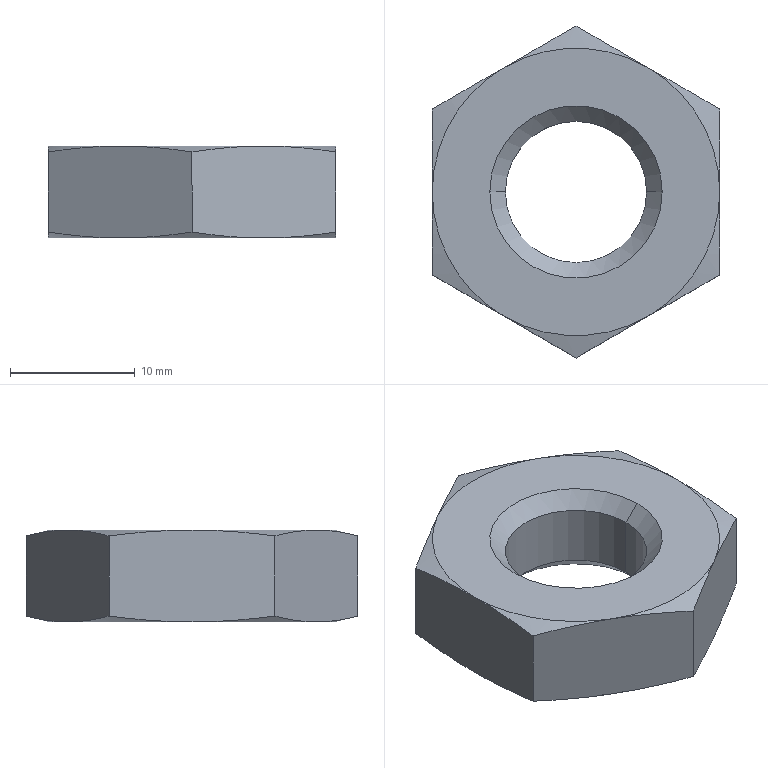Part | SolidWorks | features BaseBody 1 | 1 solid | 26 faces | box 23.077 x 26.647 x 7.385 mm | volume 2587 mm3 | cone 16 | plane 8 | cylinder 2 | commonest cylinder face diameters 11.347 x2
STEP:
#1=CARTESIAN_POINT('',(-12.08,360.269,293.557));
#2=VERTEX_POINT('',#1);
#3=CARTESIAN_POINT('',(-23.427,360.269,293.557));
#4=VERTEX_POINT('',#3);
#5=CARTESIAN_POINT('',(-17.753,360.269,293.557));
#6=DIRECTION('',(0.,0.,-1.));
#7=DIRECTION('',(0.,1.,0.));
#8=AXIS2_PLACEMENT_3D('',#5,#6,#7);
#9=CIRCLE('',#8,5.673);
#10=EDGE_CURVE('',#2,#4,#9,.T.);
#11=ORIENTED_EDGE('',*,*,#10,.F.);
#12=CARTESIAN_POINT('',(-10.83,360.269,292.308));
#13=VERTEX_POINT('',#12);
#14=CARTESIAN_POINT('',(-10.83,360.269,292.308));
#15=DIRECTION('',(0.7071,0.,-0.7071));
#16=VECTOR('',#15,1000.);
#17=LINE('',#14,#16);
#18=EDGE_CURVE('',#2,#13,#17,.T.);
#19=ORIENTED_EDGE('',*,*,#18,.T.);
#20=CARTESIAN_POINT('',(-24.677,360.269,292.308));
#21=VERTEX_POINT('',#20);
#22=CARTESIAN_POINT('',(-17.753,360.269,292.308));
#23=DIRECTION('',(0.,0.,-1.));
#24=DIRECTION('',(-1.,0.,0.));
#25=AXIS2_PLACEMENT_3D('',#22,#23,#24);
#26=CIRCLE('',#25,6.923);
#27=EDGE_CURVE('',#13,#21,#26,.T.);
#28=ORIENTED_EDGE('',*,*,#27,.T.);
#29=CARTESIAN_POINT('',(-24.677,360.269,292.308));
#30=DIRECTION('',(-0.7071,0.,-0.7071));
#31=VECTOR('',#30,1000.);
#32=LINE('',#29,#31);
#33=EDGE_CURVE('',#4,#21,#32,.T.);
#34=ORIENTED_EDGE('',*,*,#33,.F.);
#35=EDGE_LOOP('',(#11,#19,#28,#34));
#36=FACE_OUTER_BOUND('',#35,.T.);
#37=CARTESIAN_POINT('',(-17.753,360.269,292.308));
#38=DIRECTION('',(0.,0.,-1.));
#39=DIRECTION('',(-1.,0.,0.));
#40=AXIS2_PLACEMENT_3D('',#37,#38,#39);
#41=CONICAL_SURFACE('',#40,6.923,0.7854);
#42=ADVANCED_FACE('',(#36),#41,.F.);
#43=CARTESIAN_POINT('',(-12.08,360.269,298.443));
#44=VERTEX_POINT('',#43);
#45=CARTESIAN_POINT('',(-23.427,360.269,298.443));
#46=VERTEX_POINT('',#45);
#47=CARTESIAN_POINT('',(-17.753,360.269,298.443));
#48=DIRECTION('',(0.,0.,-1.));
#49=DIRECTION('',(-1.,0.,0.));
#50=AXIS2_PLACEMENT_3D('',#47,#48,#49);
#51=CIRCLE('',#50,5.673);
#52=EDGE_CURVE('',#44,#46,#51,.T.);
#53=ORIENTED_EDGE('',*,*,#52,.F.);
#54=CARTESIAN_POINT('',(-12.08,360.269,299.692));
#55=DIRECTION('',(0.,0.,-1.));
#56=VECTOR('',#55,1000.);
#57=LINE('',#54,#56);
#58=EDGE_CURVE('',#44,#2,#57,.T.);
#59=ORIENTED_EDGE('',*,*,#58,.T.);
#60=ORIENTED_EDGE('',*,*,#10,.T.);
#61=CARTESIAN_POINT('',(-23.427,360.269,299.692));
#62=DIRECTION('',(0.,0.,-1.));
#63=VECTOR('',#62,1000.);
#64=LINE('',#61,#63);
#65=EDGE_CURVE('',#46,#4,#64,.T.);
#66=ORIENTED_EDGE('',*,*,#65,.F.);
#67=EDGE_LOOP('',(#53,#59,#60,#66));
#68=FACE_OUTER_BOUND('',#67,.T.);
#69=CARTESIAN_POINT('',(-17.753,360.269,299.692));
#70=DIRECTION('',(0.,0.,-1.));
#71=DIRECTION('',(-1.,0.,0.));
#72=AXIS2_PLACEMENT_3D('',#69,#70,#71);
#73=CYLINDRICAL_SURFACE('',#72,5.673);
#74=ADVANCED_FACE('',(#68),#73,.F.);
#75=ORIENTED_EDGE('',*,*,#52,.T.);
#76=CARTESIAN_POINT('',(-24.677,360.269,299.692));
#77=VERTEX_POINT('',#76);
#78=CARTESIAN_POINT('',(-24.677,360.269,299.692));
#79=DIRECTION('',(-0.7071,0.,0.7071));
#80=VECTOR('',#79,1000.);
#81=LINE('',#78,#80);
#82=EDGE_CURVE('',#46,#77,#81,.T.);
#83=ORIENTED_EDGE('',*,*,#82,.T.);
#84=CARTESIAN_POINT('',(-10.83,360.269,299.692));
#85=VERTEX_POINT('',#84);
#86=CARTESIAN_POINT('',(-17.753,360.269,299.692));
#87=DIRECTION('',(0.,0.,-1.));
#88=DIRECTION('',(1.,0.,0.));
#89=AXIS2_PLACEMENT_3D('',#86,#87,#88);
#90=CIRCLE('',#89,6.923);
#91=EDGE_CURVE('',#85,#77,#90,.T.);
#92=ORIENTED_EDGE('',*,*,#91,.F.);
#93=CARTESIAN_POINT('',(-10.83,360.269,299.692));
#94=DIRECTION('',(0.7071,0.,0.7071));
#95=VECTOR('',#94,1000.);
#96=LINE('',#93,#95);
#97=EDGE_CURVE('',#44,#85,#96,.T.);
#98=ORIENTED_EDGE('',*,*,#97,.F.);
#99=EDGE_LOOP('',(#75,#83,#92,#98));
#100=FACE_OUTER_BOUND('',#99,.T.);
#101=CARTESIAN_POINT('',(-17.753,360.269,299.692));
#102=DIRECTION('',(0.,0.,1.));
#103=DIRECTION('',(1.,0.,0.));
#104=AXIS2_PLACEMENT_3D('',#101,#102,#103);
#105=CONICAL_SURFACE('',#104,6.923,0.7854);
#106=ADVANCED_FACE('',(#100),#105,.F.);
#107=CARTESIAN_POINT('',(-17.753,360.269,292.308));
#108=DIRECTION('',(0.,0.,-1.));
#109=DIRECTION('',(-1.,0.,0.));
#110=AXIS2_PLACEMENT_3D('',#107,#108,#109);
#111=CIRCLE('',#110,6.923);
#112=EDGE_CURVE('',#21,#13,#111,.T.);
#113=ORIENTED_EDGE('',*,*,#112,.F.);
#114=ORIENTED_EDGE('',*,*,#27,.F.);
#115=EDGE_LOOP('',(#113,#114));
#116=FACE_BOUND('',#115,.T.);
#117=CARTESIAN_POINT('',(-11.984,370.262,292.308));
#118=VERTEX_POINT('',#117);
#119=CARTESIAN_POINT('',(-23.523,370.262,292.308));
#120=VERTEX_POINT('',#119);
#121=CARTESIAN_POINT('',(-17.753,360.269,292.308));
#122=DIRECTION('',(0.,0.,1.));
#123=DIRECTION('',(1.,0.,0.));
#124=AXIS2_PLACEMENT_3D('',#121,#122,#123);
#125=CIRCLE('',#124,11.538);
#126=EDGE_CURVE('',#118,#120,#125,.T.);
#127=ORIENTED_EDGE('',*,*,#126,.F.);
#128=CARTESIAN_POINT('',(-6.215,360.269,292.308));
#129=VERTEX_POINT('',#128);
#130=CARTESIAN_POINT('',(-17.753,360.269,292.308));
#131=DIRECTION('',(0.,0.,1.));
#132=DIRECTION('',(1.,0.,0.));
#133=AXIS2_PLACEMENT_3D('',#130,#131,#132);
#134=CIRCLE('',#133,11.538);
#135=EDGE_CURVE('',#129,#118,#134,.T.);
#136=ORIENTED_EDGE('',*,*,#135,.F.);
#137=CARTESIAN_POINT('',(-11.984,350.277,292.308));
#138=VERTEX_POINT('',#137);
#139=CARTESIAN_POINT('',(-17.753,360.269,292.308));
#140=DIRECTION('',(0.,0.,1.));
#141=DIRECTION('',(1.,0.,0.));
#142=AXIS2_PLACEMENT_3D('',#139,#140,#141);
#143=CIRCLE('',#142,11.538);
#144=EDGE_CURVE('',#138,#129,#143,.T.);
#145=ORIENTED_EDGE('',*,*,#144,.F.);
#146=CARTESIAN_POINT('',(-23.523,350.277,292.308));
#147=VERTEX_POINT('',#146);
#148=CARTESIAN_POINT('',(-17.753,360.269,292.308));
#149=DIRECTION('',(0.,0.,1.));
#150=DIRECTION('',(1.,0.,0.));
#151=AXIS2_PLACEMENT_3D('',#148,#149,#150);
#152=CIRCLE('',#151,11.538);
#153=EDGE_CURVE('',#147,#138,#152,.T.);
#154=ORIENTED_EDGE('',*,*,#153,.F.);
#155=CARTESIAN_POINT('',(-29.292,360.269,292.308));
#156=VERTEX_POINT('',#155);
#157=CARTESIAN_POINT('',(-17.753,360.269,292.308));
#158=DIRECTION('',(0.,0.,1.));
#159=DIRECTION('',(1.,0.,0.));
#160=AXIS2_PLACEMENT_3D('',#157,#158,#159);
#161=CIRCLE('',#160,11.538);
#162=EDGE_CURVE('',#156,#147,#161,.T.);
#163=ORIENTED_EDGE('',*,*,#162,.F.);
#164=CARTESIAN_POINT('',(-17.753,360.269,292.308));
#165=DIRECTION('',(0.,0.,1.));
#166=DIRECTION('',(1.,0.,0.));
#167=AXIS2_PLACEMENT_3D('',#164,#165,#166);
#168=CIRCLE('',#167,11.538);
#169=EDGE_CURVE('',#120,#156,#168,.T.);
#170=ORIENTED_EDGE('',*,*,#169,.F.);
#171=EDGE_LOOP('',(#127,#136,#145,#154,#163,#170));
#172=FACE_OUTER_BOUND('',#171,.T.);
#173=CARTESIAN_POINT('',(-17.753,360.269,292.308));
#174=DIRECTION('',(0.,0.,1.));
#175=DIRECTION('',(1.,0.,0.));
#176=AXIS2_PLACEMENT_3D('',#173,#174,#175);
#177=PLANE('',#176);
#178=ADVANCED_FACE('',(#116,#172),#177,.F.);
#179=ORIENTED_EDGE('',*,*,#18,.F.);
#180=CARTESIAN_POINT('',(-17.753,360.269,293.557));
#181=DIRECTION('',(0.,0.,-1.));
#182=DIRECTION('',(0.,1.,0.));
#183=AXIS2_PLACEMENT_3D('',#180,#181,#182);
#184=CIRCLE('',#183,5.673);
#185=EDGE_CURVE('',#4,#2,#184,.T.);
#186=ORIENTED_EDGE('',*,*,#185,.F.);
#187=ORIENTED_EDGE('',*,*,#33,.T.);
#188=ORIENTED_EDGE('',*,*,#112,.T.);
#189=EDGE_LOOP('',(#179,#186,#187,#188));
#190=FACE_OUTER_BOUND('',#189,.T.);
#191=CARTESIAN_POINT('',(-17.753,360.269,292.308));
#192=DIRECTION('',(0.,0.,-1.));
#193=DIRECTION('',(-1.,0.,0.));
#194=AXIS2_PLACEMENT_3D('',#191,#192,#193);
#195=CONICAL_SURFACE('',#194,6.923,0.7854);
#196=ADVANCED_FACE('',(#190),#195,.F.);
#197=CARTESIAN_POINT('',(-17.753,373.593,292.786));
#198=VERTEX_POINT('',#197);
#199=CARTESIAN_POINT('',(-23.523,370.262,292.308));
#200=CARTESIAN_POINT('',(-22.556,370.82,292.308));
#201=CARTESIAN_POINT('',(-21.592,371.376,292.352));
#202=CARTESIAN_POINT('',(-19.67,372.486,292.517));
#203=CARTESIAN_POINT('',(-18.711,373.04,292.638));
#204=CARTESIAN_POINT('',(-17.753,373.593,292.786));
#205=B_SPLINE_CURVE_WITH_KNOTS('',3,(#199,#200,#201,#202,#203,#204),.UNSPECIFIED.,.F.,.F.,(4,2,4),(0.,0.003339,0.006679),.UNSPECIFIED.);
#206=EDGE_CURVE('',#120,#198,#205,.T.);
#207=ORIENTED_EDGE('',*,*,#206,.T.);
#208=CARTESIAN_POINT('',(-17.753,373.593,292.786));
#209=CARTESIAN_POINT('',(-16.796,373.04,292.638));
#210=CARTESIAN_POINT('',(-15.837,372.486,292.517));
#211=CARTESIAN_POINT('',(-13.914,371.376,292.352));
#212=CARTESIAN_POINT('',(-12.951,370.82,292.308));
#213=CARTESIAN_POINT('',(-11.984,370.262,292.308));
#214=B_SPLINE_CURVE_WITH_KNOTS('',3,(#208,#209,#210,#211,#212,#213),.UNSPECIFIED.,.F.,.F.,(4,2,4),(0.,0.003339,0.006679),.UNSPECIFIED.);
#215=EDGE_CURVE('',#198,#118,#214,.T.);
#216=ORIENTED_EDGE('',*,*,#215,.T.);
#217=ORIENTED_EDGE('',*,*,#126,.T.);
#218=EDGE_LOOP('',(#207,#216,#217));
#219=FACE_OUTER_BOUND('',#218,.T.);
#220=CARTESIAN_POINT('',(-17.753,360.269,292.789));
#221=DIRECTION('',(0.,0.,1.));
#222=DIRECTION('',(1.,0.,0.));
#223=AXIS2_PLACEMENT_3D('',#220,#221,#222);
#224=CONICAL_SURFACE('',#223,13.334,1.309);
#225=ADVANCED_FACE('',(#219),#224,.T.);
#226=ORIENTED_EDGE('',*,*,#135,.T.);
#227=CARTESIAN_POINT('',(-6.215,366.931,292.786));
#228=VERTEX_POINT('',#227);
#229=CARTESIAN_POINT('',(-11.984,370.262,292.308));
#230=CARTESIAN_POINT('',(-11.018,369.704,292.308));
#231=CARTESIAN_POINT('',(-10.054,369.147,292.352));
#232=CARTESIAN_POINT('',(-8.131,368.037,292.517));
#233=CARTESIAN_POINT('',(-7.172,367.484,292.638));
#234=CARTESIAN_POINT('',(-6.215,366.931,292.786));
#235=B_SPLINE_CURVE_WITH_KNOTS('',3,(#229,#230,#231,#232,#233,#234),.UNSPECIFIED.,.F.,.F.,(4,2,4),(0.,0.003339,0.006679),.UNSPECIFIED.);
#236=EDGE_CURVE('',#118,#228,#235,.T.);
#237=ORIENTED_EDGE('',*,*,#236,.T.);
#238=CARTESIAN_POINT('',(-6.215,366.931,292.786));
#239=CARTESIAN_POINT('',(-6.215,365.826,292.638));
#240=CARTESIAN_POINT('',(-6.215,364.718,292.517));
#241=CARTESIAN_POINT('',(-6.215,362.498,292.352));
#242=CARTESIAN_POINT('',(-6.215,361.385,292.308));
#243=CARTESIAN_POINT('',(-6.215,360.269,292.308));
#244=B_SPLINE_CURVE_WITH_KNOTS('',3,(#238,#239,#240,#241,#242,#243),.UNSPECIFIED.,.F.,.F.,(4,2,4),(0.,0.003339,0.006679),.UNSPECIFIED.);
#245=EDGE_CURVE('',#228,#129,#244,.T.);
#246=ORIENTED_EDGE('',*,*,#245,.T.);
#247=EDGE_LOOP('',(#226,#237,#246));
#248=FACE_OUTER_BOUND('',#247,.T.);
#249=CARTESIAN_POINT('',(-17.753,360.269,292.789));
#250=DIRECTION('',(0.,0.,1.));
#251=DIRECTION('',(1.,0.,0.));
#252=AXIS2_PLACEMENT_3D('',#249,#250,#251);
#253=CONICAL_SURFACE('',#252,13.334,1.309);
#254=ADVANCED_FACE('',(#248),#253,.T.);
#255=CARTESIAN_POINT('',(-6.215,353.607,292.786));
#256=VERTEX_POINT('',#255);
#257=CARTESIAN_POINT('',(-6.215,360.269,292.308));
#258=CARTESIAN_POINT('',(-6.215,359.153,292.308));
#259=CARTESIAN_POINT('',(-6.215,358.04,292.352));
#260=CARTESIAN_POINT('',(-6.215,355.82,292.517));
#261=CARTESIAN_POINT('',(-6.215,354.713,292.638));
#262=CARTESIAN_POINT('',(-6.215,353.607,292.786));
#263=B_SPLINE_CURVE_WITH_KNOTS('',3,(#257,#258,#259,#260,#261,#262),.UNSPECIFIED.,.F.,.F.,(4,2,4),(0.,0.003339,0.006679),.UNSPECIFIED.);
#264=EDGE_CURVE('',#129,#256,#263,.T.);
#265=ORIENTED_EDGE('',*,*,#264,.T.);
#266=CARTESIAN_POINT('',(-6.215,353.607,292.786));
#267=CARTESIAN_POINT('',(-7.172,353.055,292.638));
#268=CARTESIAN_POINT('',(-8.131,352.501,292.517));
#269=CARTESIAN_POINT('',(-10.054,351.391,292.352));
#270=CARTESIAN_POINT('',(-11.018,350.835,292.308));
#271=CARTESIAN_POINT('',(-11.984,350.277,292.308));
#272=B_SPLINE_CURVE_WITH_KNOTS('',3,(#266,#267,#268,#269,#270,#271),.UNSPECIFIED.,.F.,.F.,(4,2,4),(0.,0.003339,0.006679),.UNSPECIFIED.);
#273=EDGE_CURVE('',#256,#138,#272,.T.);
#274=ORIENTED_EDGE('',*,*,#273,.T.);
#275=ORIENTED_EDGE('',*,*,#144,.T.);
#276=EDGE_LOOP('',(#265,#274,#275));
#277=FACE_OUTER_BOUND('',#276,.T.);
#278=CARTESIAN_POINT('',(-17.753,360.269,292.789));
#279=DIRECTION('',(0.,0.,1.));
#280=DIRECTION('',(1.,0.,0.));
#281=AXIS2_PLACEMENT_3D('',#278,#279,#280);
#282=CONICAL_SURFACE('',#281,13.334,1.309);
#283=ADVANCED_FACE('',(#277),#282,.T.);
#284=CARTESIAN_POINT('',(-17.753,346.946,292.786));
#285=VERTEX_POINT('',#284);
#286=CARTESIAN_POINT('',(-11.984,350.277,292.308));
#287=CARTESIAN_POINT('',(-12.951,349.719,292.308));
#288=CARTESIAN_POINT('',(-13.914,349.162,292.352));
#289=CARTESIAN_POINT('',(-15.837,348.052,292.517));
#290=CARTESIAN_POINT('',(-16.796,347.498,292.638));
#291=CARTESIAN_POINT('',(-17.753,346.946,292.786));
#292=B_SPLINE_CURVE_WITH_KNOTS('',3,(#286,#287,#288,#289,#290,#291),.UNSPECIFIED.,.F.,.F.,(4,2,4),(0.,0.003339,0.006679),.UNSPECIFIED.);
#293=EDGE_CURVE('',#138,#285,#292,.T.);
#294=ORIENTED_EDGE('',*,*,#293,.T.);
#295=CARTESIAN_POINT('',(-17.753,346.946,292.786));
#296=CARTESIAN_POINT('',(-18.711,347.498,292.638));
#297=CARTESIAN_POINT('',(-19.67,348.052,292.517));
#298=CARTESIAN_POINT('',(-21.592,349.162,292.352));
#299=CARTESIAN_POINT('',(-22.556,349.719,292.308));
#300=CARTESIAN_POINT('',(-23.523,350.277,292.308));
#301=B_SPLINE_CURVE_WITH_KNOTS('',3,(#295,#296,#297,#298,#299,#300),.UNSPECIFIED.,.F.,.F.,(4,2,4),(0.,0.003339,0.006679),.UNSPECIFIED.);
#302=EDGE_CURVE('',#285,#147,#301,.T.);
#303=ORIENTED_EDGE('',*,*,#302,.T.);
#304=ORIENTED_EDGE('',*,*,#153,.T.);
#305=EDGE_LOOP('',(#294,#303,#304));
#306=FACE_OUTER_BOUND('',#305,.T.);
#307=CARTESIAN_POINT('',(-17.753,360.269,292.789));
#308=DIRECTION('',(0.,0.,1.));
#309=DIRECTION('',(1.,0.,0.));
#310=AXIS2_PLACEMENT_3D('',#307,#308,#309);
#311=CONICAL_SURFACE('',#310,13.334,1.309);
#312=ADVANCED_FACE('',(#306),#311,.T.);
#313=CARTESIAN_POINT('',(-29.292,353.607,292.786));
#314=VERTEX_POINT('',#313);
#315=CARTESIAN_POINT('',(-23.523,350.277,292.308));
#316=CARTESIAN_POINT('',(-24.489,350.835,292.308));
#317=CARTESIAN_POINT('',(-25.453,351.391,292.352));
#318=CARTESIAN_POINT('',(-27.376,352.501,292.517));
#319=CARTESIAN_POINT('',(-28.335,353.055,292.638));
#320=CARTESIAN_POINT('',(-29.292,353.607,292.786));
#321=B_SPLINE_CURVE_WITH_KNOTS('',3,(#315,#316,#317,#318,#319,#320),.UNSPECIFIED.,.F.,.F.,(4,2,4),(0.,0.003339,0.006679),.UNSPECIFIED.);
#322=EDGE_CURVE('',#147,#314,#321,.T.);
#323=ORIENTED_EDGE('',*,*,#322,.T.);
#324=CARTESIAN_POINT('',(-29.292,353.607,292.786));
#325=CARTESIAN_POINT('',(-29.292,354.713,292.638));
#326=CARTESIAN_POINT('',(-29.292,355.82,292.517));
#327=CARTESIAN_POINT('',(-29.292,358.04,292.352));
#328=CARTESIAN_POINT('',(-29.292,359.153,292.308));
#329=CARTESIAN_POINT('',(-29.292,360.269,292.308));
#330=B_SPLINE_CURVE_WITH_KNOTS('',3,(#324,#325,#326,#327,#328,#329),.UNSPECIFIED.,.F.,.F.,(4,2,4),(0.,0.003339,0.006679),.UNSPECIFIED.);
#331=EDGE_CURVE('',#314,#156,#330,.T.);
#332=ORIENTED_EDGE('',*,*,#331,.T.);
#333=ORIENTED_EDGE('',*,*,#162,.T.);
#334=EDGE_LOOP('',(#323,#332,#333));
#335=FACE_OUTER_BOUND('',#334,.T.);
#336=CARTESIAN_POINT('',(-17.753,360.269,292.789));
#337=DIRECTION('',(0.,0.,1.));
#338=DIRECTION('',(1.,0.,0.));
#339=AXIS2_PLACEMENT_3D('',#336,#337,#338);
#340=CONICAL_SURFACE('',#339,13.334,1.309);
#341=ADVANCED_FACE('',(#335),#340,.T.);
#342=ORIENTED_EDGE('',*,*,#169,.T.);
#343=CARTESIAN_POINT('',(-29.292,366.931,292.786));
#344=VERTEX_POINT('',#343);
#345=CARTESIAN_POINT('',(-29.292,360.269,292.308));
#346=CARTESIAN_POINT('',(-29.292,361.385,292.308));
#347=CARTESIAN_POINT('',(-29.292,362.498,292.352));
#348=CARTESIAN_POINT('',(-29.292,364.718,292.517));
#349=CARTESIAN_POINT('',(-29.292,365.826,292.638));
#350=CARTESIAN_POINT('',(-29.292,366.931,292.786));
#351=B_SPLINE_CURVE_WITH_KNOTS('',3,(#345,#346,#347,#348,#349,#350),.UNSPECIFIED.,.F.,.F.,(4,2,4),(0.,0.003339,0.006679),.UNSPECIFIED.);
#352=EDGE_CURVE('',#156,#344,#351,.T.);
#353=ORIENTED_EDGE('',*,*,#352,.T.);
#354=CARTESIAN_POINT('',(-29.292,366.931,292.786));
#355=CARTESIAN_POINT('',(-28.335,367.484,292.638));
#356=CARTESIAN_POINT('',(-27.376,368.037,292.517));
#357=CARTESIAN_POINT('',(-25.453,369.147,292.352));
#358=CARTESIAN_POINT('',(-24.489,369.704,292.308));
#359=CARTESIAN_POINT('',(-23.523,370.262,292.308));
#360=B_SPLINE_CURVE_WITH_KNOTS('',3,(#354,#355,#356,#357,#358,#359),.UNSPECIFIED.,.F.,.F.,(4,2,4),(0.,0.003339,0.006679),.UNSPECIFIED.);
#361=EDGE_CURVE('',#344,#120,#360,.T.);
#362=ORIENTED_EDGE('',*,*,#361,.T.);
#363=EDGE_LOOP('',(#342,#353,#362));
#364=FACE_OUTER_BOUND('',#363,.T.);
#365=CARTESIAN_POINT('',(-17.753,360.269,292.789));
#366=DIRECTION('',(0.,0.,1.));
#367=DIRECTION('',(1.,0.,0.));
#368=AXIS2_PLACEMENT_3D('',#365,#366,#367);
#369=CONICAL_SURFACE('',#368,13.334,1.309);
#370=ADVANCED_FACE('',(#364),#369,.T.);
#371=ORIENTED_EDGE('',*,*,#58,.F.);
#372=CARTESIAN_POINT('',(-17.753,360.269,298.443));
#373=DIRECTION('',(0.,0.,-1.));
#374=DIRECTION('',(-1.,0.,0.));
#375=AXIS2_PLACEMENT_3D('',#372,#373,#374);
#376=CIRCLE('',#375,5.673);
#377=EDGE_CURVE('',#46,#44,#376,.T.);
#378=ORIENTED_EDGE('',*,*,#377,.F.);
#379=ORIENTED_EDGE('',*,*,#65,.T.);
#380=ORIENTED_EDGE('',*,*,#185,.T.);
#381=EDGE_LOOP('',(#371,#378,#379,#380));
#382=FACE_OUTER_BOUND('',#381,.T.);
#383=CARTESIAN_POINT('',(-17.753,360.269,299.692));
#384=DIRECTION('',(0.,0.,-1.));
#385=DIRECTION('',(-1.,0.,0.));
#386=AXIS2_PLACEMENT_3D('',#383,#384,#385);
#387=CYLINDRICAL_SURFACE('',#386,5.673);
#388=ADVANCED_FACE('',(#382),#387,.F.);
#389=CARTESIAN_POINT('',(-17.753,373.593,299.214));
#390=VERTEX_POINT('',#389);
#391=CARTESIAN_POINT('',(-17.753,373.593,282.615));
#392=DIRECTION('',(0.,0.,1.));
#393=VECTOR('',#392,1000.);
#394=LINE('',#391,#393);
#395=EDGE_CURVE('',#198,#390,#394,.T.);
#396=ORIENTED_EDGE('',*,*,#395,.F.);
#397=ORIENTED_EDGE('',*,*,#206,.F.);
#398=ORIENTED_EDGE('',*,*,#361,.F.);
#399=CARTESIAN_POINT('',(-29.292,366.931,299.214));
#400=VERTEX_POINT('',#399);
#401=CARTESIAN_POINT('',(-29.292,366.931,282.615));
#402=DIRECTION('',(0.,0.,-1.));
#403=VECTOR('',#402,1000.);
#404=LINE('',#401,#403);
#405=EDGE_CURVE('',#400,#344,#404,.T.);
#406=ORIENTED_EDGE('',*,*,#405,.F.);
#407=CARTESIAN_POINT('',(-23.523,370.262,299.692));
#408=VERTEX_POINT('',#407);
#409=CARTESIAN_POINT('',(-23.523,370.262,299.692));
#410=CARTESIAN_POINT('',(-24.489,369.704,299.692));
#411=CARTESIAN_POINT('',(-25.453,369.147,299.648));
#412=CARTESIAN_POINT('',(-27.376,368.037,299.483));
#413=CARTESIAN_POINT('',(-28.335,367.484,299.362));
#414=CARTESIAN_POINT('',(-29.292,366.931,299.214));
#415=B_SPLINE_CURVE_WITH_KNOTS('',3,(#409,#410,#411,#412,#413,#414),.UNSPECIFIED.,.F.,.F.,(4,2,4),(0.,0.003339,0.006679),.UNSPECIFIED.);
#416=EDGE_CURVE('',#408,#400,#415,.T.);
#417=ORIENTED_EDGE('',*,*,#416,.F.);
#418=CARTESIAN_POINT('',(-17.753,373.593,299.214));
#419=CARTESIAN_POINT('',(-18.711,373.04,299.362));
#420=CARTESIAN_POINT('',(-19.67,372.486,299.483));
#421=CARTESIAN_POINT('',(-21.592,371.376,299.648));
#422=CARTESIAN_POINT('',(-22.556,370.82,299.692));
#423=CARTESIAN_POINT('',(-23.523,370.262,299.692));
#424=B_SPLINE_CURVE_WITH_KNOTS('',3,(#418,#419,#420,#421,#422,#423),.UNSPECIFIED.,.F.,.F.,(4,2,4),(0.,0.003339,0.006679),.UNSPECIFIED.);
#425=EDGE_CURVE('',#390,#408,#424,.T.);
#426=ORIENTED_EDGE('',*,*,#425,.F.);
#427=EDGE_LOOP('',(#396,#397,#398,#406,#417,#426));
#428=FACE_OUTER_BOUND('',#427,.T.);
#429=CARTESIAN_POINT('',(-29.292,366.931,282.615));
#430=DIRECTION('',(0.5,-0.866,0.));
#431=DIRECTION('',(0.866,0.5,0.));
#432=AXIS2_PLACEMENT_3D('',#429,#430,#431);
#433=PLANE('',#432);
#434=ADVANCED_FACE('',(#428),#433,.F.);
#435=CARTESIAN_POINT('',(-6.215,366.931,299.214));
#436=VERTEX_POINT('',#435);
#437=CARTESIAN_POINT('',(-6.215,366.931,282.615));
#438=DIRECTION('',(0.,0.,1.));
#439=VECTOR('',#438,1000.);
#440=LINE('',#437,#439);
#441=EDGE_CURVE('',#228,#436,#440,.T.);
#442=ORIENTED_EDGE('',*,*,#441,.F.);
#443=ORIENTED_EDGE('',*,*,#236,.F.);
#444=ORIENTED_EDGE('',*,*,#215,.F.);
#445=ORIENTED_EDGE('',*,*,#395,.T.);
#446=CARTESIAN_POINT('',(-11.984,370.262,299.692));
#447=VERTEX_POINT('',#446);
#448=CARTESIAN_POINT('',(-11.984,370.262,299.692));
#449=CARTESIAN_POINT('',(-12.951,370.82,299.692));
#450=CARTESIAN_POINT('',(-13.914,371.376,299.648));
#451=CARTESIAN_POINT('',(-15.837,372.486,299.483));
#452=CARTESIAN_POINT('',(-16.796,373.04,299.362));
#453=CARTESIAN_POINT('',(-17.753,373.593,299.214));
#454=B_SPLINE_CURVE_WITH_KNOTS('',3,(#448,#449,#450,#451,#452,#453),.UNSPECIFIED.,.F.,.F.,(4,2,4),(0.,0.003339,0.006679),.UNSPECIFIED.);
#455=EDGE_CURVE('',#447,#390,#454,.T.);
#456=ORIENTED_EDGE('',*,*,#455,.F.);
#457=CARTESIAN_POINT('',(-6.215,366.931,299.214));
#458=CARTESIAN_POINT('',(-7.172,367.484,299.362));
#459=CARTESIAN_POINT('',(-8.131,368.037,299.483));
#460=CARTESIAN_POINT('',(-10.054,369.147,299.648));
#461=CARTESIAN_POINT('',(-11.018,369.704,299.692));
#462=CARTESIAN_POINT('',(-11.984,370.262,299.692));
#463=B_SPLINE_CURVE_WITH_KNOTS('',3,(#457,#458,#459,#460,#461,#462),.UNSPECIFIED.,.F.,.F.,(4,2,4),(0.,0.003339,0.006679),.UNSPECIFIED.);
#464=EDGE_CURVE('',#436,#447,#463,.T.);
#465=ORIENTED_EDGE('',*,*,#464,.F.);
#466=EDGE_LOOP('',(#442,#443,#444,#445,#456,#465));
#467=FACE_OUTER_BOUND('',#466,.T.);
#468=CARTESIAN_POINT('',(-17.753,373.593,282.615));
#469=DIRECTION('',(-0.5,-0.866,0.));
#470=DIRECTION('',(0.866,-0.5,0.));
#471=AXIS2_PLACEMENT_3D('',#468,#469,#470);
#472=PLANE('',#471);
#473=ADVANCED_FACE('',(#467),#472,.F.);
#474=CARTESIAN_POINT('',(-6.215,353.607,299.214));
#475=VERTEX_POINT('',#474);
#476=CARTESIAN_POINT('',(-6.215,353.607,282.615));
#477=DIRECTION('',(0.,0.,1.));
#478=VECTOR('',#477,1000.);
#479=LINE('',#476,#478);
#480=EDGE_CURVE('',#256,#475,#479,.T.);
#481=ORIENTED_EDGE('',*,*,#480,.F.);
#482=ORIENTED_EDGE('',*,*,#264,.F.);
#483=ORIENTED_EDGE('',*,*,#245,.F.);
#484=ORIENTED_EDGE('',*,*,#441,.T.);
#485=CARTESIAN_POINT('',(-6.215,360.269,299.692));
#486=VERTEX_POINT('',#485);
#487=CARTESIAN_POINT('',(-6.215,360.269,299.692));
#488=CARTESIAN_POINT('',(-6.215,361.385,299.692));
#489=CARTESIAN_POINT('',(-6.215,362.498,299.648));
#490=CARTESIAN_POINT('',(-6.215,364.718,299.483));
#491=CARTESIAN_POINT('',(-6.215,365.826,299.362));
#492=CARTESIAN_POINT('',(-6.215,366.931,299.214));
#493=B_SPLINE_CURVE_WITH_KNOTS('',3,(#487,#488,#489,#490,#491,#492),.UNSPECIFIED.,.F.,.F.,(4,2,4),(0.,0.003339,0.006679),.UNSPECIFIED.);
#494=EDGE_CURVE('',#486,#436,#493,.T.);
#495=ORIENTED_EDGE('',*,*,#494,.F.);
#496=CARTESIAN_POINT('',(-6.215,353.607,299.214));
#497=CARTESIAN_POINT('',(-6.215,354.713,299.362));
#498=CARTESIAN_POINT('',(-6.215,355.82,299.483));
#499=CARTESIAN_POINT('',(-6.215,358.04,299.648));
#500=CARTESIAN_POINT('',(-6.215,359.153,299.692));
#501=CARTESIAN_POINT('',(-6.215,360.269,299.692));
#502=B_SPLINE_CURVE_WITH_KNOTS('',3,(#496,#497,#498,#499,#500,#501),.UNSPECIFIED.,.F.,.F.,(4,2,4),(0.,0.003339,0.006679),.UNSPECIFIED.);
#503=EDGE_CURVE('',#475,#486,#502,.T.);
#504=ORIENTED_EDGE('',*,*,#503,.F.);
#505=EDGE_LOOP('',(#481,#482,#483,#484,#495,#504));
#506=FACE_OUTER_BOUND('',#505,.T.);
#507=CARTESIAN_POINT('',(-6.215,366.931,282.615));
#508=DIRECTION('',(-1.,0.,0.));
#509=DIRECTION('',(0.,0.,1.));
#510=AXIS2_PLACEMENT_3D('',#507,#508,#509);
#511=PLANE('',#510);
#512=ADVANCED_FACE('',(#506),#511,.F.);
#513=CARTESIAN_POINT('',(-17.753,346.946,299.214));
#514=VERTEX_POINT('',#513);
#515=CARTESIAN_POINT('',(-17.753,346.946,282.615));
#516=DIRECTION('',(0.,0.,1.));
#517=VECTOR('',#516,1000.);
#518=LINE('',#515,#517);
#519=EDGE_CURVE('',#285,#514,#518,.T.);
#520=ORIENTED_EDGE('',*,*,#519,.F.);
#521=ORIENTED_EDGE('',*,*,#293,.F.);
#522=ORIENTED_EDGE('',*,*,#273,.F.);
#523=ORIENTED_EDGE('',*,*,#480,.T.);
#524=CARTESIAN_POINT('',(-11.984,350.277,299.692));
#525=VERTEX_POINT('',#524);
#526=CARTESIAN_POINT('',(-11.984,350.277,299.692));
#527=CARTESIAN_POINT('',(-11.018,350.835,299.692));
#528=CARTESIAN_POINT('',(-10.054,351.391,299.648));
#529=CARTESIAN_POINT('',(-8.131,352.501,299.483));
#530=CARTESIAN_POINT('',(-7.172,353.055,299.362));
#531=CARTESIAN_POINT('',(-6.215,353.607,299.214));
#532=B_SPLINE_CURVE_WITH_KNOTS('',3,(#526,#527,#528,#529,#530,#531),.UNSPECIFIED.,.F.,.F.,(4,2,4),(0.,0.003339,0.006679),.UNSPECIFIED.);
#533=EDGE_CURVE('',#525,#475,#532,.T.);
#534=ORIENTED_EDGE('',*,*,#533,.F.);
#535=CARTESIAN_POINT('',(-17.753,346.946,299.214));
#536=CARTESIAN_POINT('',(-16.796,347.498,299.362));
#537=CARTESIAN_POINT('',(-15.837,348.052,299.483));
#538=CARTESIAN_POINT('',(-13.914,349.162,299.648));
#539=CARTESIAN_POINT('',(-12.951,349.719,299.692));
#540=CARTESIAN_POINT('',(-11.984,350.277,299.692));
#541=B_SPLINE_CURVE_WITH_KNOTS('',3,(#535,#536,#537,#538,#539,#540),.UNSPECIFIED.,.F.,.F.,(4,2,4),(0.,0.003339,0.006679),.UNSPECIFIED.);
#542=EDGE_CURVE('',#514,#525,#541,.T.);
#543=ORIENTED_EDGE('',*,*,#542,.F.);
#544=EDGE_LOOP('',(#520,#521,#522,#523,#534,#543));
#545=FACE_OUTER_BOUND('',#544,.T.);
#546=CARTESIAN_POINT('',(-6.215,353.607,282.615));
#547=DIRECTION('',(-0.5,0.866,0.));
#548=DIRECTION('',(-0.866,-0.5,0.));
#549=AXIS2_PLACEMENT_3D('',#546,#547,#548);
#550=PLANE('',#549);
#551=ADVANCED_FACE('',(#545),#550,.F.);
#552=CARTESIAN_POINT('',(-29.292,353.607,299.214));
#553=VERTEX_POINT('',#552);
#554=CARTESIAN_POINT('',(-29.292,353.607,282.615));
#555=DIRECTION('',(0.,0.,1.));
#556=VECTOR('',#555,1000.);
#557=LINE('',#554,#556);
#558=EDGE_CURVE('',#314,#553,#557,.T.);
#559=ORIENTED_EDGE('',*,*,#558,.F.);
#560=ORIENTED_EDGE('',*,*,#322,.F.);
#561=ORIENTED_EDGE('',*,*,#302,.F.);
#562=ORIENTED_EDGE('',*,*,#519,.T.);
#563=CARTESIAN_POINT('',(-23.523,350.277,299.692));
#564=VERTEX_POINT('',#563);
#565=CARTESIAN_POINT('',(-23.523,350.277,299.692));
#566=CARTESIAN_POINT('',(-22.556,349.719,299.692));
#567=CARTESIAN_POINT('',(-21.592,349.162,299.648));
#568=CARTESIAN_POINT('',(-19.67,348.052,299.483));
#569=CARTESIAN_POINT('',(-18.711,347.498,299.362));
#570=CARTESIAN_POINT('',(-17.753,346.946,299.214));
#571=B_SPLINE_CURVE_WITH_KNOTS('',3,(#565,#566,#567,#568,#569,#570),.UNSPECIFIED.,.F.,.F.,(4,2,4),(0.,0.003339,0.006679),.UNSPECIFIED.);
#572=EDGE_CURVE('',#564,#514,#571,.T.);
#573=ORIENTED_EDGE('',*,*,#572,.F.);
#574=CARTESIAN_POINT('',(-29.292,353.607,299.214));
#575=CARTESIAN_POINT('',(-28.335,353.055,299.362));
#576=CARTESIAN_POINT('',(-27.376,352.501,299.483));
#577=CARTESIAN_POINT('',(-25.453,351.391,299.648));
#578=CARTESIAN_POINT('',(-24.489,350.835,299.692));
#579=CARTESIAN_POINT('',(-23.523,350.277,299.692));
#580=B_SPLINE_CURVE_WITH_KNOTS('',3,(#574,#575,#576,#577,#578,#579),.UNSPECIFIED.,.F.,.F.,(4,2,4),(0.,0.003339,0.006679),.UNSPECIFIED.);
#581=EDGE_CURVE('',#553,#564,#580,.T.);
#582=ORIENTED_EDGE('',*,*,#581,.F.);
#583=EDGE_LOOP('',(#559,#560,#561,#562,#573,#582));
#584=FACE_OUTER_BOUND('',#583,.T.);
#585=CARTESIAN_POINT('',(-17.753,346.946,282.615));
#586=DIRECTION('',(0.5,0.866,0.));
#587=DIRECTION('',(-0.866,0.5,0.));
#588=AXIS2_PLACEMENT_3D('',#585,#586,#587);
#589=PLANE('',#588);
#590=ADVANCED_FACE('',(#584),#589,.F.);
#591=ORIENTED_EDGE('',*,*,#405,.T.);
#592=ORIENTED_EDGE('',*,*,#352,.F.);
#593=ORIENTED_EDGE('',*,*,#331,.F.);
#594=ORIENTED_EDGE('',*,*,#558,.T.);
#595=CARTESIAN_POINT('',(-29.292,360.269,299.692));
#596=VERTEX_POINT('',#595);
#597=CARTESIAN_POINT('',(-29.292,360.269,299.692));
#598=CARTESIAN_POINT('',(-29.292,359.153,299.692));
#599=CARTESIAN_POINT('',(-29.292,358.04,299.648));
#600=CARTESIAN_POINT('',(-29.292,355.82,299.483));
#601=CARTESIAN_POINT('',(-29.292,354.713,299.362));
#602=CARTESIAN_POINT('',(-29.292,353.607,299.214));
#603=B_SPLINE_CURVE_WITH_KNOTS('',3,(#597,#598,#599,#600,#601,#602),.UNSPECIFIED.,.F.,.F.,(4,2,4),(0.,0.003339,0.006679),.UNSPECIFIED.);
#604=EDGE_CURVE('',#596,#553,#603,.T.);
#605=ORIENTED_EDGE('',*,*,#604,.F.);
#606=CARTESIAN_POINT('',(-29.292,366.931,299.214));
#607=CARTESIAN_POINT('',(-29.292,365.826,299.362));
#608=CARTESIAN_POINT('',(-29.292,364.718,299.483));
#609=CARTESIAN_POINT('',(-29.292,362.498,299.648));
#610=CARTESIAN_POINT('',(-29.292,361.385,299.692));
#611=CARTESIAN_POINT('',(-29.292,360.269,299.692));
#612=B_SPLINE_CURVE_WITH_KNOTS('',3,(#606,#607,#608,#609,#610,#611),.UNSPECIFIED.,.F.,.F.,(4,2,4),(0.,0.003339,0.006679),.UNSPECIFIED.);
#613=EDGE_CURVE('',#400,#596,#612,.T.);
#614=ORIENTED_EDGE('',*,*,#613,.F.);
#615=EDGE_LOOP('',(#591,#592,#593,#594,#605,#614));
#616=FACE_OUTER_BOUND('',#615,.T.);
#617=CARTESIAN_POINT('',(-29.292,353.607,282.615));
#618=DIRECTION('',(1.,0.,0.));
#619=DIRECTION('',(0.,0.,-1.));
#620=AXIS2_PLACEMENT_3D('',#617,#618,#619);
#621=PLANE('',#620);
#622=ADVANCED_FACE('',(#616),#621,.F.);
#623=ORIENTED_EDGE('',*,*,#82,.F.);
#624=ORIENTED_EDGE('',*,*,#377,.T.);
#625=ORIENTED_EDGE('',*,*,#97,.T.);
#626=CARTESIAN_POINT('',(-17.753,360.269,299.692));
#627=DIRECTION('',(0.,0.,-1.));
#628=DIRECTION('',(1.,0.,0.));
#629=AXIS2_PLACEMENT_3D('',#626,#627,#628);
#630=CIRCLE('',#629,6.923);
#631=EDGE_CURVE('',#77,#85,#630,.T.);
#632=ORIENTED_EDGE('',*,*,#631,.F.);
#633=EDGE_LOOP('',(#623,#624,#625,#632));
#634=FACE_OUTER_BOUND('',#633,.T.);
#635=CARTESIAN_POINT('',(-17.753,360.269,299.692));
#636=DIRECTION('',(0.,0.,1.));
#637=DIRECTION('',(1.,0.,0.));
#638=AXIS2_PLACEMENT_3D('',#635,#636,#637);
#639=CONICAL_SURFACE('',#638,6.923,0.7854);
#640=ADVANCED_FACE('',(#634),#639,.F.);
#641=CARTESIAN_POINT('',(-17.753,360.269,299.692));
#642=DIRECTION('',(0.,0.,-1.));
#643=DIRECTION('',(-1.,0.,0.));
#644=AXIS2_PLACEMENT_3D('',#641,#642,#643);
#645=CIRCLE('',#644,11.538);
#646=EDGE_CURVE('',#408,#447,#645,.T.);
#647=ORIENTED_EDGE('',*,*,#646,.T.);
#648=ORIENTED_EDGE('',*,*,#455,.T.);
#649=ORIENTED_EDGE('',*,*,#425,.T.);
#650=EDGE_LOOP('',(#647,#648,#649));
#651=FACE_OUTER_BOUND('',#650,.T.);
#652=CARTESIAN_POINT('',(-17.753,360.269,299.211));
#653=DIRECTION('',(0.,0.,-1.));
#654=DIRECTION('',(-1.,0.,0.));
#655=AXIS2_PLACEMENT_3D('',#652,#653,#654);
#656=CONICAL_SURFACE('',#655,13.334,1.309);
#657=ADVANCED_FACE('',(#651),#656,.T.);
#658=CARTESIAN_POINT('',(-17.753,360.269,299.692));
#659=DIRECTION('',(0.,0.,-1.));
#660=DIRECTION('',(-1.,0.,0.));
#661=AXIS2_PLACEMENT_3D('',#658,#659,#660);
#662=CIRCLE('',#661,11.538);
#663=EDGE_CURVE('',#596,#408,#662,.T.);
#664=ORIENTED_EDGE('',*,*,#663,.T.);
#665=ORIENTED_EDGE('',*,*,#416,.T.);
#666=ORIENTED_EDGE('',*,*,#613,.T.);
#667=EDGE_LOOP('',(#664,#665,#666));
#668=FACE_OUTER_BOUND('',#667,.T.);
#669=CARTESIAN_POINT('',(-17.753,360.269,299.211));
#670=DIRECTION('',(0.,0.,-1.));
#671=DIRECTION('',(-1.,0.,0.));
#672=AXIS2_PLACEMENT_3D('',#669,#670,#671);
#673=CONICAL_SURFACE('',#672,13.334,1.309);
#674=ADVANCED_FACE('',(#668),#673,.T.);
#675=ORIENTED_EDGE('',*,*,#494,.T.);
#676=ORIENTED_EDGE('',*,*,#464,.T.);
#677=CARTESIAN_POINT('',(-17.753,360.269,299.692));
#678=DIRECTION('',(0.,0.,-1.));
#679=DIRECTION('',(0.,1.,0.));
#680=AXIS2_PLACEMENT_3D('',#677,#678,#679);
#681=CIRCLE('',#680,11.538);
#682=EDGE_CURVE('',#447,#486,#681,.T.);
#683=ORIENTED_EDGE('',*,*,#682,.T.);
#684=EDGE_LOOP('',(#675,#676,#683));
#685=FACE_OUTER_BOUND('',#684,.T.);
#686=CARTESIAN_POINT('',(-17.753,360.269,299.211));
#687=DIRECTION('',(0.,0.,-1.));
#688=DIRECTION('',(0.,1.,0.));
#689=AXIS2_PLACEMENT_3D('',#686,#687,#688);
#690=CONICAL_SURFACE('',#689,13.334,1.309);
#691=ADVANCED_FACE('',(#685),#690,.T.);
#692=CARTESIAN_POINT('',(-17.753,360.269,299.692));
#693=DIRECTION('',(0.,0.,-1.));
#694=DIRECTION('',(-1.,0.,0.));
#695=AXIS2_PLACEMENT_3D('',#692,#693,#694);
#696=CIRCLE('',#695,11.538);
#697=EDGE_CURVE('',#486,#525,#696,.T.);
#698=ORIENTED_EDGE('',*,*,#697,.T.);
#699=ORIENTED_EDGE('',*,*,#533,.T.);
#700=ORIENTED_EDGE('',*,*,#503,.T.);
#701=EDGE_LOOP('',(#698,#699,#700));
#702=FACE_OUTER_BOUND('',#701,.T.);
#703=CARTESIAN_POINT('',(-17.753,360.269,299.211));
#704=DIRECTION('',(0.,0.,-1.));
#705=DIRECTION('',(-1.,0.,0.));
#706=AXIS2_PLACEMENT_3D('',#703,#704,#705);
#707=CONICAL_SURFACE('',#706,13.334,1.309);
#708=ADVANCED_FACE('',(#702),#707,.T.);
#709=CARTESIAN_POINT('',(-17.753,360.269,299.692));
#710=DIRECTION('',(0.,0.,-1.));
#711=DIRECTION('',(-1.,0.,0.));
#712=AXIS2_PLACEMENT_3D('',#709,#710,#711);
#713=CIRCLE('',#712,11.538);
#714=EDGE_CURVE('',#525,#564,#713,.T.);
#715=ORIENTED_EDGE('',*,*,#714,.T.);
#716=ORIENTED_EDGE('',*,*,#572,.T.);
#717=ORIENTED_EDGE('',*,*,#542,.T.);
#718=EDGE_LOOP('',(#715,#716,#717));
#719=FACE_OUTER_BOUND('',#718,.T.);
#720=CARTESIAN_POINT('',(-17.753,360.269,299.211));
#721=DIRECTION('',(0.,0.,-1.));
#722=DIRECTION('',(-1.,0.,0.));
#723=AXIS2_PLACEMENT_3D('',#720,#721,#722);
#724=CONICAL_SURFACE('',#723,13.334,1.309);
#725=ADVANCED_FACE('',(#719),#724,.T.);
#726=CARTESIAN_POINT('',(-17.753,360.269,299.692));
#727=DIRECTION('',(0.,0.,-1.));
#728=DIRECTION('',(0.,1.,0.));
#729=AXIS2_PLACEMENT_3D('',#726,#727,#728);
#730=CIRCLE('',#729,11.538);
#731=EDGE_CURVE('',#564,#596,#730,.T.);
#732=ORIENTED_EDGE('',*,*,#731,.T.);
#733=ORIENTED_EDGE('',*,*,#604,.T.);
#734=ORIENTED_EDGE('',*,*,#581,.T.);
#735=EDGE_LOOP('',(#732,#733,#734));
#736=FACE_OUTER_BOUND('',#735,.T.);
#737=CARTESIAN_POINT('',(-17.753,360.269,299.211));
#738=DIRECTION('',(0.,0.,-1.));
#739=DIRECTION('',(0.,1.,0.));
#740=AXIS2_PLACEMENT_3D('',#737,#738,#739);
#741=CONICAL_SURFACE('',#740,13.334,1.309);
#742=ADVANCED_FACE('',(#736),#741,.T.);
#743=ORIENTED_EDGE('',*,*,#91,.T.);
#744=ORIENTED_EDGE('',*,*,#631,.T.);
#745=EDGE_LOOP('',(#743,#744));
#746=FACE_BOUND('',#745,.T.);
#747=ORIENTED_EDGE('',*,*,#697,.F.);
#748=ORIENTED_EDGE('',*,*,#682,.F.);
#749=ORIENTED_EDGE('',*,*,#646,.F.);
#750=ORIENTED_EDGE('',*,*,#663,.F.);
#751=ORIENTED_EDGE('',*,*,#731,.F.);
#752=ORIENTED_EDGE('',*,*,#714,.F.);
#753=EDGE_LOOP('',(#747,#748,#749,#750,#751,#752));
#754=FACE_OUTER_BOUND('',#753,.T.);
#755=CARTESIAN_POINT('',(-29.292,360.269,299.692));
#756=DIRECTION('',(0.,0.,-1.));
#757=DIRECTION('',(-1.,0.,0.));
#758=AXIS2_PLACEMENT_3D('',#755,#756,#757);
#759=PLANE('',#758);
#760=ADVANCED_FACE('',(#746,#754),#759,.F.);
#761=CLOSED_SHELL('',(#42,#74,#106,#178,#196,#225,#254,#283,#312,#341,#370,#388,#434,#473,#512,#551,#590,#622,#640,#657,#674,#691,#708,#725,#742,#760));
#762=MANIFOLD_SOLID_BREP('',#761);
#763=CARTESIAN_POINT('',(0.,0.,0.));
#764=DIRECTION('',(0.,0.,1.));
#765=DIRECTION('',(1.,0.,0.));
#766=AXIS2_PLACEMENT_3D('',#763,#764,#765);
#767=(LENGTH_UNIT()NAMED_UNIT(*)SI_UNIT(.MILLI.,.METRE.));
#768=UNCERTAINTY_MEASURE_WITH_UNIT(LENGTH_MEASURE(0.00001),#767,'','');
#769=(NAMED_UNIT(*)PLANE_ANGLE_UNIT()SI_UNIT($,.RADIAN.));
#770=(NAMED_UNIT(*)SI_UNIT($,.STERADIAN.)SOLID_ANGLE_UNIT());
#771=(GEOMETRIC_REPRESENTATION_CONTEXT(3)GLOBAL_UNCERTAINTY_ASSIGNED_CONTEXT((#768))GLOBAL_UNIT_ASSIGNED_CONTEXT((#767,#769,#770))REPRESENTATION_CONTEXT('',''));
#772=ADVANCED_BREP_SHAPE_REPRESENTATION('',(#762,#766),#771);